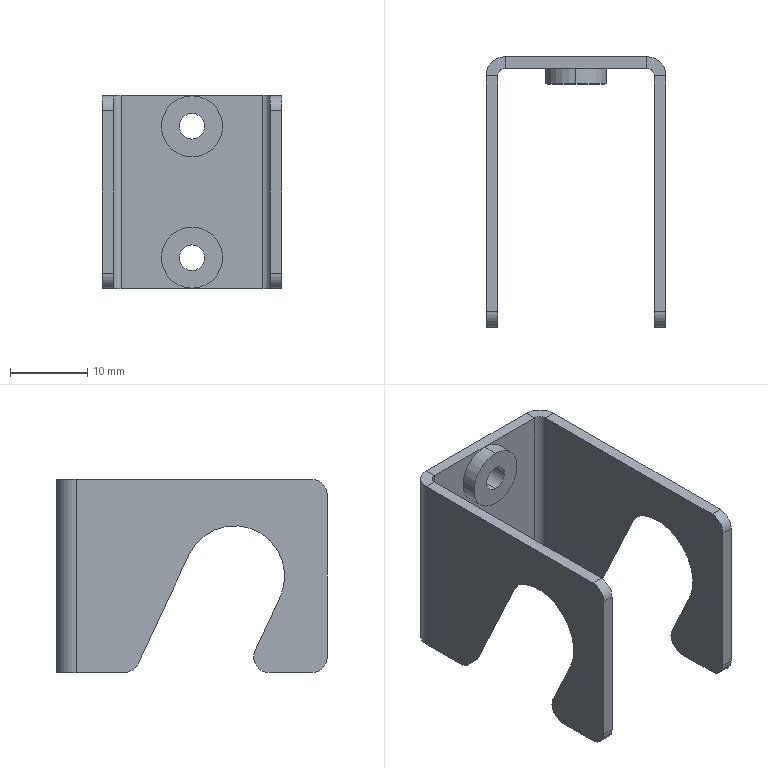Part | SolidWorks | features BaseBody 1 | 1 solid | 48 faces | box 23.3 x 35 x 25 mm | volume 2716 mm3 | plane 26 | cylinder 22 | commonest cylinder face diameters 4 x8 3.3 x4 7.9 x4 2 x2 5 x2 13 x2
STEP:
#1=CARTESIAN_POINT('',(0.,0.,10.15));
#2=VERTEX_POINT('',#1);
#3=CARTESIAN_POINT('',(0.,-3.5,10.15));
#4=VERTEX_POINT('',#3);
#5=CARTESIAN_POINT('',(0.,-3.5,10.15));
#6=DIRECTION('',(0.,-1.,0.));
#7=VECTOR('',#6,1000.);
#8=LINE('',#5,#7);
#9=EDGE_CURVE('',#2,#4,#8,.T.);
#10=ORIENTED_EDGE('',*,*,#9,.F.);
#11=CARTESIAN_POINT('',(0.,0.,6.85));
#12=VERTEX_POINT('',#11);
#13=CARTESIAN_POINT('',(0.,0.,8.5));
#14=DIRECTION('',(0.,-1.,0.));
#15=DIRECTION('',(0.,0.,-1.));
#16=AXIS2_PLACEMENT_3D('',#13,#14,#15);
#17=CIRCLE('',#16,1.65);
#18=EDGE_CURVE('',#12,#2,#17,.T.);
#19=ORIENTED_EDGE('',*,*,#18,.F.);
#20=CARTESIAN_POINT('',(0.,-3.5,6.85));
#21=VERTEX_POINT('',#20);
#22=CARTESIAN_POINT('',(0.,-3.5,6.85));
#23=DIRECTION('',(0.,-1.,0.));
#24=VECTOR('',#23,1000.);
#25=LINE('',#22,#24);
#26=EDGE_CURVE('',#12,#21,#25,.T.);
#27=ORIENTED_EDGE('',*,*,#26,.T.);
#28=CARTESIAN_POINT('',(0.,-3.5,8.5));
#29=DIRECTION('',(0.,-1.,0.));
#30=DIRECTION('',(0.,0.,-1.));
#31=AXIS2_PLACEMENT_3D('',#28,#29,#30);
#32=CIRCLE('',#31,1.65);
#33=EDGE_CURVE('',#21,#4,#32,.T.);
#34=ORIENTED_EDGE('',*,*,#33,.T.);
#35=EDGE_LOOP('',(#10,#19,#27,#34));
#36=FACE_OUTER_BOUND('',#35,.T.);
#37=CARTESIAN_POINT('',(0.,-3.5,8.5));
#38=DIRECTION('',(0.,-1.,0.));
#39=DIRECTION('',(0.,0.,-1.));
#40=AXIS2_PLACEMENT_3D('',#37,#38,#39);
#41=CYLINDRICAL_SURFACE('',#40,1.65);
#42=ADVANCED_FACE('',(#36),#41,.F.);
#43=CARTESIAN_POINT('',(0.,0.,-6.85));
#44=VERTEX_POINT('',#43);
#45=CARTESIAN_POINT('',(0.,-3.5,-6.85));
#46=VERTEX_POINT('',#45);
#47=CARTESIAN_POINT('',(0.,-3.5,-6.85));
#48=DIRECTION('',(0.,-1.,0.));
#49=VECTOR('',#48,1000.);
#50=LINE('',#47,#49);
#51=EDGE_CURVE('',#44,#46,#50,.T.);
#52=ORIENTED_EDGE('',*,*,#51,.F.);
#53=CARTESIAN_POINT('',(0.,0.,-10.15));
#54=VERTEX_POINT('',#53);
#55=CARTESIAN_POINT('',(0.,0.,-8.5));
#56=DIRECTION('',(0.,-1.,0.));
#57=DIRECTION('',(0.,0.,-1.));
#58=AXIS2_PLACEMENT_3D('',#55,#56,#57);
#59=CIRCLE('',#58,1.65);
#60=EDGE_CURVE('',#54,#44,#59,.T.);
#61=ORIENTED_EDGE('',*,*,#60,.F.);
#62=CARTESIAN_POINT('',(0.,-3.5,-10.15));
#63=VERTEX_POINT('',#62);
#64=CARTESIAN_POINT('',(0.,-3.5,-10.15));
#65=DIRECTION('',(0.,-1.,0.));
#66=VECTOR('',#65,1000.);
#67=LINE('',#64,#66);
#68=EDGE_CURVE('',#54,#63,#67,.T.);
#69=ORIENTED_EDGE('',*,*,#68,.T.);
#70=CARTESIAN_POINT('',(0.,-3.5,-8.5));
#71=DIRECTION('',(0.,-1.,0.));
#72=DIRECTION('',(0.,0.,-1.));
#73=AXIS2_PLACEMENT_3D('',#70,#71,#72);
#74=CIRCLE('',#73,1.65);
#75=EDGE_CURVE('',#63,#46,#74,.T.);
#76=ORIENTED_EDGE('',*,*,#75,.T.);
#77=EDGE_LOOP('',(#52,#61,#69,#76));
#78=FACE_OUTER_BOUND('',#77,.T.);
#79=CARTESIAN_POINT('',(0.,-3.5,-8.5));
#80=DIRECTION('',(0.,-1.,0.));
#81=DIRECTION('',(0.,0.,-1.));
#82=AXIS2_PLACEMENT_3D('',#79,#80,#81);
#83=CYLINDRICAL_SURFACE('',#82,1.65);
#84=ADVANCED_FACE('',(#78),#83,.F.);
#85=CARTESIAN_POINT('',(0.,-3.5,-12.45));
#86=VERTEX_POINT('',#85);
#87=CARTESIAN_POINT('',(0.,-1.5,-12.45));
#88=VERTEX_POINT('',#87);
#89=CARTESIAN_POINT('',(0.,-3.5,-12.45));
#90=DIRECTION('',(0.,1.,0.));
#91=VECTOR('',#90,1000.);
#92=LINE('',#89,#91);
#93=EDGE_CURVE('',#86,#88,#92,.T.);
#94=ORIENTED_EDGE('',*,*,#93,.F.);
#95=CARTESIAN_POINT('',(0.,-3.5,-4.55));
#96=VERTEX_POINT('',#95);
#97=CARTESIAN_POINT('',(0.,-3.5,-8.5));
#98=DIRECTION('',(0.,-1.,0.));
#99=DIRECTION('',(0.,0.,1.));
#100=AXIS2_PLACEMENT_3D('',#97,#98,#99);
#101=CIRCLE('',#100,3.95);
#102=EDGE_CURVE('',#96,#86,#101,.T.);
#103=ORIENTED_EDGE('',*,*,#102,.F.);
#104=CARTESIAN_POINT('',(0.,-1.5,-4.55));
#105=VERTEX_POINT('',#104);
#106=CARTESIAN_POINT('',(0.,-3.5,-4.55));
#107=DIRECTION('',(0.,1.,0.));
#108=VECTOR('',#107,1000.);
#109=LINE('',#106,#108);
#110=EDGE_CURVE('',#96,#105,#109,.T.);
#111=ORIENTED_EDGE('',*,*,#110,.T.);
#112=CARTESIAN_POINT('',(0.,-1.5,-8.5));
#113=DIRECTION('',(0.,-1.,0.));
#114=DIRECTION('',(0.,0.,1.));
#115=AXIS2_PLACEMENT_3D('',#112,#113,#114);
#116=CIRCLE('',#115,3.95);
#117=EDGE_CURVE('',#105,#88,#116,.T.);
#118=ORIENTED_EDGE('',*,*,#117,.T.);
#119=EDGE_LOOP('',(#94,#103,#111,#118));
#120=FACE_OUTER_BOUND('',#119,.T.);
#121=CARTESIAN_POINT('',(0.,-3.5,-8.5));
#122=DIRECTION('',(0.,1.,0.));
#123=DIRECTION('',(0.,0.,1.));
#124=AXIS2_PLACEMENT_3D('',#121,#122,#123);
#125=CYLINDRICAL_SURFACE('',#124,3.95);
#126=ADVANCED_FACE('',(#120),#125,.T.);
#127=ORIENTED_EDGE('',*,*,#33,.F.);
#128=CARTESIAN_POINT('',(0.,-3.5,8.5));
#129=DIRECTION('',(0.,-1.,0.));
#130=DIRECTION('',(0.,0.,-1.));
#131=AXIS2_PLACEMENT_3D('',#128,#129,#130);
#132=CIRCLE('',#131,1.65);
#133=EDGE_CURVE('',#4,#21,#132,.T.);
#134=ORIENTED_EDGE('',*,*,#133,.F.);
#135=EDGE_LOOP('',(#127,#134));
#136=FACE_BOUND('',#135,.T.);
#137=CARTESIAN_POINT('',(0.,-3.5,12.45));
#138=VERTEX_POINT('',#137);
#139=CARTESIAN_POINT('',(0.,-3.5,4.55));
#140=VERTEX_POINT('',#139);
#141=CARTESIAN_POINT('',(0.,-3.5,8.5));
#142=DIRECTION('',(0.,-1.,0.));
#143=DIRECTION('',(0.,0.,-1.));
#144=AXIS2_PLACEMENT_3D('',#141,#142,#143);
#145=CIRCLE('',#144,3.95);
#146=EDGE_CURVE('',#138,#140,#145,.T.);
#147=ORIENTED_EDGE('',*,*,#146,.T.);
#148=CARTESIAN_POINT('',(0.,-3.5,8.5));
#149=DIRECTION('',(0.,-1.,0.));
#150=DIRECTION('',(0.,0.,-1.));
#151=AXIS2_PLACEMENT_3D('',#148,#149,#150);
#152=CIRCLE('',#151,3.95);
#153=EDGE_CURVE('',#140,#138,#152,.T.);
#154=ORIENTED_EDGE('',*,*,#153,.T.);
#155=EDGE_LOOP('',(#147,#154));
#156=FACE_OUTER_BOUND('',#155,.T.);
#157=CARTESIAN_POINT('',(0.,-3.5,8.5));
#158=DIRECTION('',(0.,-1.,0.));
#159=DIRECTION('',(0.,0.,-1.));
#160=AXIS2_PLACEMENT_3D('',#157,#158,#159);
#161=PLANE('',#160);
#162=ADVANCED_FACE('',(#136,#156),#161,.T.);
#163=CARTESIAN_POINT('',(0.,-1.5,4.55));
#164=VERTEX_POINT('',#163);
#165=CARTESIAN_POINT('',(0.,-3.5,4.55));
#166=DIRECTION('',(0.,1.,0.));
#167=VECTOR('',#166,1000.);
#168=LINE('',#165,#167);
#169=EDGE_CURVE('',#140,#164,#168,.T.);
#170=ORIENTED_EDGE('',*,*,#169,.F.);
#171=ORIENTED_EDGE('',*,*,#146,.F.);
#172=CARTESIAN_POINT('',(0.,-1.5,12.45));
#173=VERTEX_POINT('',#172);
#174=CARTESIAN_POINT('',(0.,-3.5,12.45));
#175=DIRECTION('',(0.,1.,0.));
#176=VECTOR('',#175,1000.);
#177=LINE('',#174,#176);
#178=EDGE_CURVE('',#138,#173,#177,.T.);
#179=ORIENTED_EDGE('',*,*,#178,.T.);
#180=CARTESIAN_POINT('',(0.,-1.5,8.5));
#181=DIRECTION('',(0.,-1.,0.));
#182=DIRECTION('',(0.,0.,1.));
#183=AXIS2_PLACEMENT_3D('',#180,#181,#182);
#184=CIRCLE('',#183,3.95);
#185=EDGE_CURVE('',#173,#164,#184,.T.);
#186=ORIENTED_EDGE('',*,*,#185,.T.);
#187=EDGE_LOOP('',(#170,#171,#179,#186));
#188=FACE_OUTER_BOUND('',#187,.T.);
#189=CARTESIAN_POINT('',(0.,-3.5,8.5));
#190=DIRECTION('',(0.,1.,0.));
#191=DIRECTION('',(0.,0.,1.));
#192=AXIS2_PLACEMENT_3D('',#189,#190,#191);
#193=CYLINDRICAL_SURFACE('',#192,3.95);
#194=ADVANCED_FACE('',(#188),#193,.T.);
#195=CARTESIAN_POINT('',(11.65,-27.483,-12.5));
#196=VERTEX_POINT('',#195);
#197=CARTESIAN_POINT('',(11.65,-25.67,-9.655));
#198=VERTEX_POINT('',#197);
#199=CARTESIAN_POINT('',(11.65,-27.483,-10.5));
#200=DIRECTION('',(1.,0.,0.));
#201=DIRECTION('',(0.,1.,0.));
#202=AXIS2_PLACEMENT_3D('',#199,#200,#201);
#203=CIRCLE('',#202,2.);
#204=EDGE_CURVE('',#196,#198,#203,.T.);
#205=ORIENTED_EDGE('',*,*,#204,.F.);
#206=CARTESIAN_POINT('',(10.15,-27.483,-12.5));
#207=VERTEX_POINT('',#206);
#208=CARTESIAN_POINT('',(11.65,-27.483,-12.5));
#209=DIRECTION('',(1.,0.,0.));
#210=VECTOR('',#209,1000.);
#211=LINE('',#208,#210);
#212=EDGE_CURVE('',#207,#196,#211,.T.);
#213=ORIENTED_EDGE('',*,*,#212,.F.);
#214=CARTESIAN_POINT('',(10.15,-25.67,-9.655));
#215=VERTEX_POINT('',#214);
#216=CARTESIAN_POINT('',(10.15,-27.483,-10.5));
#217=DIRECTION('',(-1.,0.,0.));
#218=DIRECTION('',(0.,1.,0.));
#219=AXIS2_PLACEMENT_3D('',#216,#217,#218);
#220=CIRCLE('',#219,2.);
#221=EDGE_CURVE('',#215,#207,#220,.T.);
#222=ORIENTED_EDGE('',*,*,#221,.F.);
#223=CARTESIAN_POINT('',(11.65,-25.67,-9.655));
#224=DIRECTION('',(-1.,0.,0.));
#225=VECTOR('',#224,1000.);
#226=LINE('',#223,#225);
#227=EDGE_CURVE('',#198,#215,#226,.T.);
#228=ORIENTED_EDGE('',*,*,#227,.F.);
#229=EDGE_LOOP('',(#205,#213,#222,#228));
#230=FACE_OUTER_BOUND('',#229,.T.);
#231=CARTESIAN_POINT('',(11.65,-27.483,-10.5));
#232=DIRECTION('',(-1.,0.,0.));
#233=DIRECTION('',(0.,-1.,0.));
#234=AXIS2_PLACEMENT_3D('',#231,#232,#233);
#235=CYLINDRICAL_SURFACE('',#234,2.);
#236=ADVANCED_FACE('',(#230),#235,.T.);
#237=CARTESIAN_POINT('',(-10.15,-27.483,-12.5));
#238=VERTEX_POINT('',#237);
#239=CARTESIAN_POINT('',(-10.15,-25.67,-9.655));
#240=VERTEX_POINT('',#239);
#241=CARTESIAN_POINT('',(-10.15,-27.483,-10.5));
#242=DIRECTION('',(1.,0.,0.));
#243=DIRECTION('',(0.,1.,0.));
#244=AXIS2_PLACEMENT_3D('',#241,#242,#243);
#245=CIRCLE('',#244,2.);
#246=EDGE_CURVE('',#238,#240,#245,.T.);
#247=ORIENTED_EDGE('',*,*,#246,.F.);
#248=CARTESIAN_POINT('',(-11.65,-27.483,-12.5));
#249=VERTEX_POINT('',#248);
#250=CARTESIAN_POINT('',(-11.65,-27.483,-12.5));
#251=DIRECTION('',(1.,0.,0.));
#252=VECTOR('',#251,1000.);
#253=LINE('',#250,#252);
#254=EDGE_CURVE('',#249,#238,#253,.T.);
#255=ORIENTED_EDGE('',*,*,#254,.F.);
#256=CARTESIAN_POINT('',(-11.65,-25.67,-9.655));
#257=VERTEX_POINT('',#256);
#258=CARTESIAN_POINT('',(-11.65,-27.483,-10.5));
#259=DIRECTION('',(-1.,0.,0.));
#260=DIRECTION('',(0.,1.,0.));
#261=AXIS2_PLACEMENT_3D('',#258,#259,#260);
#262=CIRCLE('',#261,2.);
#263=EDGE_CURVE('',#257,#249,#262,.T.);
#264=ORIENTED_EDGE('',*,*,#263,.F.);
#265=CARTESIAN_POINT('',(-10.15,-25.67,-9.655));
#266=DIRECTION('',(-1.,0.,0.));
#267=VECTOR('',#266,1000.);
#268=LINE('',#265,#267);
#269=EDGE_CURVE('',#240,#257,#268,.T.);
#270=ORIENTED_EDGE('',*,*,#269,.F.);
#271=EDGE_LOOP('',(#247,#255,#264,#270));
#272=FACE_OUTER_BOUND('',#271,.T.);
#273=CARTESIAN_POINT('',(-10.15,-27.483,-10.5));
#274=DIRECTION('',(-1.,0.,0.));
#275=DIRECTION('',(0.,-1.,0.));
#276=AXIS2_PLACEMENT_3D('',#273,#274,#275);
#277=CYLINDRICAL_SURFACE('',#276,2.);
#278=ADVANCED_FACE('',(#272),#277,.T.);
#279=CARTESIAN_POINT('',(-11.65,-33.,-12.5));
#280=VERTEX_POINT('',#279);
#281=CARTESIAN_POINT('',(-11.65,-35.,-10.5));
#282=VERTEX_POINT('',#281);
#283=CARTESIAN_POINT('',(-11.65,-33.,-10.5));
#284=DIRECTION('',(-1.,0.,0.));
#285=DIRECTION('',(0.,1.,0.));
#286=AXIS2_PLACEMENT_3D('',#283,#284,#285);
#287=CIRCLE('',#286,2.);
#288=EDGE_CURVE('',#280,#282,#287,.T.);
#289=ORIENTED_EDGE('',*,*,#288,.F.);
#290=CARTESIAN_POINT('',(-10.15,-33.,-12.5));
#291=VERTEX_POINT('',#290);
#292=CARTESIAN_POINT('',(-11.65,-33.,-12.5));
#293=DIRECTION('',(-1.,0.,0.));
#294=VECTOR('',#293,1000.);
#295=LINE('',#292,#294);
#296=EDGE_CURVE('',#291,#280,#295,.T.);
#297=ORIENTED_EDGE('',*,*,#296,.F.);
#298=CARTESIAN_POINT('',(-10.15,-35.,-10.5));
#299=VERTEX_POINT('',#298);
#300=CARTESIAN_POINT('',(-10.15,-33.,-10.5));
#301=DIRECTION('',(1.,0.,0.));
#302=DIRECTION('',(0.,1.,0.));
#303=AXIS2_PLACEMENT_3D('',#300,#301,#302);
#304=CIRCLE('',#303,2.);
#305=EDGE_CURVE('',#299,#291,#304,.T.);
#306=ORIENTED_EDGE('',*,*,#305,.F.);
#307=CARTESIAN_POINT('',(-11.65,-35.,-10.5));
#308=DIRECTION('',(1.,0.,0.));
#309=VECTOR('',#308,1000.);
#310=LINE('',#307,#309);
#311=EDGE_CURVE('',#282,#299,#310,.T.);
#312=ORIENTED_EDGE('',*,*,#311,.F.);
#313=EDGE_LOOP('',(#289,#297,#306,#312));
#314=FACE_OUTER_BOUND('',#313,.T.);
#315=CARTESIAN_POINT('',(-11.65,-33.,-10.5));
#316=DIRECTION('',(1.,0.,0.));
#317=DIRECTION('',(0.,1.,0.));
#318=AXIS2_PLACEMENT_3D('',#315,#316,#317);
#319=CYLINDRICAL_SURFACE('',#318,2.);
#320=ADVANCED_FACE('',(#314),#319,.T.);
#321=CARTESIAN_POINT('',(11.65,-35.,-10.5));
#322=VERTEX_POINT('',#321);
#323=CARTESIAN_POINT('',(11.65,-33.,-12.5));
#324=VERTEX_POINT('',#323);
#325=CARTESIAN_POINT('',(11.65,-33.,-10.5));
#326=DIRECTION('',(1.,0.,0.));
#327=DIRECTION('',(0.,1.,0.));
#328=AXIS2_PLACEMENT_3D('',#325,#326,#327);
#329=CIRCLE('',#328,2.);
#330=EDGE_CURVE('',#322,#324,#329,.T.);
#331=ORIENTED_EDGE('',*,*,#330,.F.);
#332=CARTESIAN_POINT('',(10.15,-35.,-10.5));
#333=VERTEX_POINT('',#332);
#334=CARTESIAN_POINT('',(11.65,-35.,-10.5));
#335=DIRECTION('',(1.,0.,0.));
#336=VECTOR('',#335,1000.);
#337=LINE('',#334,#336);
#338=EDGE_CURVE('',#333,#322,#337,.T.);
#339=ORIENTED_EDGE('',*,*,#338,.F.);
#340=CARTESIAN_POINT('',(10.15,-33.,-12.5));
#341=VERTEX_POINT('',#340);
#342=CARTESIAN_POINT('',(10.15,-33.,-10.5));
#343=DIRECTION('',(-1.,0.,0.));
#344=DIRECTION('',(0.,1.,0.));
#345=AXIS2_PLACEMENT_3D('',#342,#343,#344);
#346=CIRCLE('',#345,2.);
#347=EDGE_CURVE('',#341,#333,#346,.T.);
#348=ORIENTED_EDGE('',*,*,#347,.F.);
#349=CARTESIAN_POINT('',(11.65,-33.,-12.5));
#350=DIRECTION('',(-1.,0.,0.));
#351=VECTOR('',#350,1000.);
#352=LINE('',#349,#351);
#353=EDGE_CURVE('',#324,#341,#352,.T.);
#354=ORIENTED_EDGE('',*,*,#353,.F.);
#355=EDGE_LOOP('',(#331,#339,#348,#354));
#356=FACE_OUTER_BOUND('',#355,.T.);
#357=CARTESIAN_POINT('',(11.65,-33.,-10.5));
#358=DIRECTION('',(-1.,0.,0.));
#359=DIRECTION('',(0.,-1.,0.));
#360=AXIS2_PLACEMENT_3D('',#357,#358,#359);
#361=CYLINDRICAL_SURFACE('',#360,2.);
#362=ADVANCED_FACE('',(#356),#361,.T.);
#363=CARTESIAN_POINT('',(-11.65,-35.,10.5));
#364=VERTEX_POINT('',#363);
#365=CARTESIAN_POINT('',(-11.65,-33.,12.5));
#366=VERTEX_POINT('',#365);
#367=CARTESIAN_POINT('',(-11.65,-33.,10.5));
#368=DIRECTION('',(-1.,0.,0.));
#369=DIRECTION('',(0.,1.,0.));
#370=AXIS2_PLACEMENT_3D('',#367,#368,#369);
#371=CIRCLE('',#370,2.);
#372=EDGE_CURVE('',#364,#366,#371,.T.);
#373=ORIENTED_EDGE('',*,*,#372,.F.);
#374=CARTESIAN_POINT('',(-10.15,-35.,10.5));
#375=VERTEX_POINT('',#374);
#376=CARTESIAN_POINT('',(-11.65,-35.,10.5));
#377=DIRECTION('',(-1.,0.,0.));
#378=VECTOR('',#377,1000.);
#379=LINE('',#376,#378);
#380=EDGE_CURVE('',#375,#364,#379,.T.);
#381=ORIENTED_EDGE('',*,*,#380,.F.);
#382=CARTESIAN_POINT('',(-10.15,-33.,12.5));
#383=VERTEX_POINT('',#382);
#384=CARTESIAN_POINT('',(-10.15,-33.,10.5));
#385=DIRECTION('',(1.,0.,0.));
#386=DIRECTION('',(0.,1.,0.));
#387=AXIS2_PLACEMENT_3D('',#384,#385,#386);
#388=CIRCLE('',#387,2.);
#389=EDGE_CURVE('',#383,#375,#388,.T.);
#390=ORIENTED_EDGE('',*,*,#389,.F.);
#391=CARTESIAN_POINT('',(-11.65,-33.,12.5));
#392=DIRECTION('',(1.,0.,0.));
#393=VECTOR('',#392,1000.);
#394=LINE('',#391,#393);
#395=EDGE_CURVE('',#366,#383,#394,.T.);
#396=ORIENTED_EDGE('',*,*,#395,.F.);
#397=EDGE_LOOP('',(#373,#381,#390,#396));
#398=FACE_OUTER_BOUND('',#397,.T.);
#399=CARTESIAN_POINT('',(-11.65,-33.,10.5));
#400=DIRECTION('',(1.,0.,0.));
#401=DIRECTION('',(0.,1.,0.));
#402=AXIS2_PLACEMENT_3D('',#399,#400,#401);
#403=CYLINDRICAL_SURFACE('',#402,2.);
#404=ADVANCED_FACE('',(#398),#403,.T.);
#405=CARTESIAN_POINT('',(11.65,-33.,12.5));
#406=VERTEX_POINT('',#405);
#407=CARTESIAN_POINT('',(11.65,-35.,10.5));
#408=VERTEX_POINT('',#407);
#409=CARTESIAN_POINT('',(11.65,-33.,10.5));
#410=DIRECTION('',(1.,0.,0.));
#411=DIRECTION('',(0.,1.,0.));
#412=AXIS2_PLACEMENT_3D('',#409,#410,#411);
#413=CIRCLE('',#412,2.);
#414=EDGE_CURVE('',#406,#408,#413,.T.);
#415=ORIENTED_EDGE('',*,*,#414,.F.);
#416=CARTESIAN_POINT('',(10.15,-33.,12.5));
#417=VERTEX_POINT('',#416);
#418=CARTESIAN_POINT('',(11.65,-33.,12.5));
#419=DIRECTION('',(1.,0.,0.));
#420=VECTOR('',#419,1000.);
#421=LINE('',#418,#420);
#422=EDGE_CURVE('',#417,#406,#421,.T.);
#423=ORIENTED_EDGE('',*,*,#422,.F.);
#424=CARTESIAN_POINT('',(10.15,-35.,10.5));
#425=VERTEX_POINT('',#424);
#426=CARTESIAN_POINT('',(10.15,-33.,10.5));
#427=DIRECTION('',(-1.,0.,0.));
#428=DIRECTION('',(0.,1.,0.));
#429=AXIS2_PLACEMENT_3D('',#426,#427,#428);
#430=CIRCLE('',#429,2.);
#431=EDGE_CURVE('',#425,#417,#430,.T.);
#432=ORIENTED_EDGE('',*,*,#431,.F.);
#433=CARTESIAN_POINT('',(11.65,-35.,10.5));
#434=DIRECTION('',(-1.,0.,0.));
#435=VECTOR('',#434,1000.);
#436=LINE('',#433,#435);
#437=EDGE_CURVE('',#408,#425,#436,.T.);
#438=ORIENTED_EDGE('',*,*,#437,.F.);
#439=EDGE_LOOP('',(#415,#423,#432,#438));
#440=FACE_OUTER_BOUND('',#439,.T.);
#441=CARTESIAN_POINT('',(11.65,-33.,10.5));
#442=DIRECTION('',(-1.,0.,0.));
#443=DIRECTION('',(0.,-1.,0.));
#444=AXIS2_PLACEMENT_3D('',#441,#442,#443);
#445=CYLINDRICAL_SURFACE('',#444,2.);
#446=ADVANCED_FACE('',(#440),#445,.T.);
#447=CARTESIAN_POINT('',(-10.15,-10.538,-11.345));
#448=VERTEX_POINT('',#447);
#449=CARTESIAN_POINT('',(-10.15,-8.726,-12.5));
#450=VERTEX_POINT('',#449);
#451=CARTESIAN_POINT('',(-10.15,-8.726,-10.5));
#452=DIRECTION('',(1.,0.,0.));
#453=DIRECTION('',(0.,1.,0.));
#454=AXIS2_PLACEMENT_3D('',#451,#452,#453);
#455=CIRCLE('',#454,2.);
#456=EDGE_CURVE('',#448,#450,#455,.T.);
#457=ORIENTED_EDGE('',*,*,#456,.F.);
#458=CARTESIAN_POINT('',(-11.65,-10.538,-11.345));
#459=VERTEX_POINT('',#458);
#460=CARTESIAN_POINT('',(-10.15,-10.538,-11.345));
#461=DIRECTION('',(1.,0.,0.));
#462=VECTOR('',#461,1000.);
#463=LINE('',#460,#462);
#464=EDGE_CURVE('',#459,#448,#463,.T.);
#465=ORIENTED_EDGE('',*,*,#464,.F.);
#466=CARTESIAN_POINT('',(-11.65,-8.726,-12.5));
#467=VERTEX_POINT('',#466);
#468=CARTESIAN_POINT('',(-11.65,-8.726,-10.5));
#469=DIRECTION('',(-1.,0.,0.));
#470=DIRECTION('',(0.,1.,0.));
#471=AXIS2_PLACEMENT_3D('',#468,#469,#470);
#472=CIRCLE('',#471,2.);
#473=EDGE_CURVE('',#467,#459,#472,.T.);
#474=ORIENTED_EDGE('',*,*,#473,.F.);
#475=CARTESIAN_POINT('',(-11.65,-8.726,-12.5));
#476=DIRECTION('',(-1.,0.,0.));
#477=VECTOR('',#476,1000.);
#478=LINE('',#475,#477);
#479=EDGE_CURVE('',#450,#467,#478,.T.);
#480=ORIENTED_EDGE('',*,*,#479,.F.);
#481=EDGE_LOOP('',(#457,#465,#474,#480));
#482=FACE_OUTER_BOUND('',#481,.T.);
#483=CARTESIAN_POINT('',(-11.65,-8.726,-10.5));
#484=DIRECTION('',(-1.,0.,0.));
#485=DIRECTION('',(0.,-1.,0.));
#486=AXIS2_PLACEMENT_3D('',#483,#484,#485);
#487=CYLINDRICAL_SURFACE('',#486,2.);
#488=ADVANCED_FACE('',(#482),#487,.T.);
#489=CARTESIAN_POINT('',(11.65,-10.538,-11.345));
#490=VERTEX_POINT('',#489);
#491=CARTESIAN_POINT('',(11.65,-8.726,-12.5));
#492=VERTEX_POINT('',#491);
#493=CARTESIAN_POINT('',(11.65,-8.726,-10.5));
#494=DIRECTION('',(1.,0.,0.));
#495=DIRECTION('',(0.,1.,0.));
#496=AXIS2_PLACEMENT_3D('',#493,#494,#495);
#497=CIRCLE('',#496,2.);
#498=EDGE_CURVE('',#490,#492,#497,.T.);
#499=ORIENTED_EDGE('',*,*,#498,.F.);
#500=CARTESIAN_POINT('',(10.15,-10.538,-11.345));
#501=VERTEX_POINT('',#500);
#502=CARTESIAN_POINT('',(11.65,-10.538,-11.345));
#503=DIRECTION('',(1.,0.,0.));
#504=VECTOR('',#503,1000.);
#505=LINE('',#502,#504);
#506=EDGE_CURVE('',#501,#490,#505,.T.);
#507=ORIENTED_EDGE('',*,*,#506,.F.);
#508=CARTESIAN_POINT('',(10.15,-8.726,-12.5));
#509=VERTEX_POINT('',#508);
#510=CARTESIAN_POINT('',(10.15,-8.726,-10.5));
#511=DIRECTION('',(-1.,0.,0.));
#512=DIRECTION('',(0.,1.,0.));
#513=AXIS2_PLACEMENT_3D('',#510,#511,#512);
#514=CIRCLE('',#513,2.);
#515=EDGE_CURVE('',#509,#501,#514,.T.);
#516=ORIENTED_EDGE('',*,*,#515,.F.);
#517=CARTESIAN_POINT('',(11.65,-8.726,-12.5));
#518=DIRECTION('',(-1.,0.,0.));
#519=VECTOR('',#518,1000.);
#520=LINE('',#517,#519);
#521=EDGE_CURVE('',#492,#509,#520,.T.);
#522=ORIENTED_EDGE('',*,*,#521,.F.);
#523=EDGE_LOOP('',(#499,#507,#516,#522));
#524=FACE_OUTER_BOUND('',#523,.T.);
#525=CARTESIAN_POINT('',(11.65,-8.726,-10.5));
#526=DIRECTION('',(-1.,0.,0.));
#527=DIRECTION('',(0.,-1.,0.));
#528=AXIS2_PLACEMENT_3D('',#525,#526,#527);
#529=CYLINDRICAL_SURFACE('',#528,2.);
#530=ADVANCED_FACE('',(#524),#529,.T.);
#531=CARTESIAN_POINT('',(11.65,-28.891,-2.747));
#532=VERTEX_POINT('',#531);
#533=CARTESIAN_POINT('',(11.65,-17.109,2.747));
#534=VERTEX_POINT('',#533);
#535=CARTESIAN_POINT('',(11.65,-23.,0.));
#536=DIRECTION('',(-1.,0.,0.));
#537=DIRECTION('',(0.,1.,0.));
#538=AXIS2_PLACEMENT_3D('',#535,#536,#537);
#539=CIRCLE('',#538,6.5);
#540=EDGE_CURVE('',#532,#534,#539,.T.);
#541=ORIENTED_EDGE('',*,*,#540,.F.);
#542=CARTESIAN_POINT('',(10.15,-28.891,-2.747));
#543=VERTEX_POINT('',#542);
#544=CARTESIAN_POINT('',(11.65,-28.891,-2.747));
#545=DIRECTION('',(-1.,0.,0.));
#546=VECTOR('',#545,1000.);
#547=LINE('',#544,#546);
#548=EDGE_CURVE('',#532,#543,#547,.T.);
#549=ORIENTED_EDGE('',*,*,#548,.T.);
#550=CARTESIAN_POINT('',(10.15,-17.109,2.747));
#551=VERTEX_POINT('',#550);
#552=CARTESIAN_POINT('',(10.15,-23.,0.));
#553=DIRECTION('',(-1.,0.,0.));
#554=DIRECTION('',(0.,1.,0.));
#555=AXIS2_PLACEMENT_3D('',#552,#553,#554);
#556=CIRCLE('',#555,6.5);
#557=EDGE_CURVE('',#543,#551,#556,.T.);
#558=ORIENTED_EDGE('',*,*,#557,.T.);
#559=CARTESIAN_POINT('',(11.65,-17.109,2.747));
#560=DIRECTION('',(-1.,0.,0.));
#561=VECTOR('',#560,1000.);
#562=LINE('',#559,#561);
#563=EDGE_CURVE('',#534,#551,#562,.T.);
#564=ORIENTED_EDGE('',*,*,#563,.F.);
#565=EDGE_LOOP('',(#541,#549,#558,#564));
#566=FACE_OUTER_BOUND('',#565,.T.);
#567=CARTESIAN_POINT('',(11.65,-23.,0.));
#568=DIRECTION('',(1.,0.,0.));
#569=DIRECTION('',(0.,1.,0.));
#570=AXIS2_PLACEMENT_3D('',#567,#568,#569);
#571=CYLINDRICAL_SURFACE('',#570,6.5);
#572=ADVANCED_FACE('',(#566),#571,.F.);
#573=CARTESIAN_POINT('',(10.15,-13.002,-6.062));
#574=DIRECTION('',(0.,0.4226,-0.9063));
#575=VECTOR('',#574,1000.);
#576=LINE('',#573,#575);
#577=EDGE_CURVE('',#551,#501,#576,.T.);
#578=ORIENTED_EDGE('',*,*,#577,.T.);
#579=ORIENTED_EDGE('',*,*,#506,.T.);
#580=CARTESIAN_POINT('',(11.65,-13.002,-6.062));
#581=DIRECTION('',(0.,0.4226,-0.9063));
#582=VECTOR('',#581,1000.);
#583=LINE('',#580,#582);
#584=EDGE_CURVE('',#534,#490,#583,.T.);
#585=ORIENTED_EDGE('',*,*,#584,.F.);
#586=ORIENTED_EDGE('',*,*,#563,.T.);
#587=EDGE_LOOP('',(#578,#579,#585,#586));
#588=FACE_OUTER_BOUND('',#587,.T.);
#589=CARTESIAN_POINT('',(11.65,-13.002,-6.062));
#590=DIRECTION('',(0.,-0.9063,-0.4226));
#591=DIRECTION('',(0.,0.4226,-0.9063));
#592=AXIS2_PLACEMENT_3D('',#589,#590,#591);
#593=PLANE('',#592);
#594=ADVANCED_FACE('',(#588),#593,.T.);
#595=CARTESIAN_POINT('',(11.65,-24.784,-11.556));
#596=DIRECTION('',(0.,-0.4226,0.9063));
#597=VECTOR('',#596,1000.);
#598=LINE('',#595,#597);
#599=EDGE_CURVE('',#198,#532,#598,.T.);
#600=ORIENTED_EDGE('',*,*,#599,.F.);
#601=ORIENTED_EDGE('',*,*,#227,.T.);
#602=CARTESIAN_POINT('',(10.15,-24.784,-11.556));
#603=DIRECTION('',(0.,-0.4226,0.9063));
#604=VECTOR('',#603,1000.);
#605=LINE('',#602,#604);
#606=EDGE_CURVE('',#215,#543,#605,.T.);
#607=ORIENTED_EDGE('',*,*,#606,.T.);
#608=ORIENTED_EDGE('',*,*,#548,.F.);
#609=EDGE_LOOP('',(#600,#601,#607,#608));
#610=FACE_OUTER_BOUND('',#609,.T.);
#611=CARTESIAN_POINT('',(11.65,-24.784,-11.556));
#612=DIRECTION('',(0.,0.9063,0.4226));
#613=DIRECTION('',(1.,0.,0.));
#614=AXIS2_PLACEMENT_3D('',#611,#612,#613);
#615=PLANE('',#614);
#616=ADVANCED_FACE('',(#610),#615,.T.);
#617=CARTESIAN_POINT('',(-10.15,-28.891,-2.747));
#618=VERTEX_POINT('',#617);
#619=CARTESIAN_POINT('',(-10.15,-24.784,-11.556));
#620=DIRECTION('',(0.,-0.4226,0.9063));
#621=VECTOR('',#620,1000.);
#622=LINE('',#619,#621);
#623=EDGE_CURVE('',#240,#618,#622,.T.);
#624=ORIENTED_EDGE('',*,*,#623,.F.);
#625=ORIENTED_EDGE('',*,*,#269,.T.);
#626=CARTESIAN_POINT('',(-11.65,-28.891,-2.747));
#627=VERTEX_POINT('',#626);
#628=CARTESIAN_POINT('',(-11.65,-24.784,-11.556));
#629=DIRECTION('',(0.,-0.4226,0.9063));
#630=VECTOR('',#629,1000.);
#631=LINE('',#628,#630);
#632=EDGE_CURVE('',#257,#627,#631,.T.);
#633=ORIENTED_EDGE('',*,*,#632,.T.);
#634=CARTESIAN_POINT('',(-10.15,-28.891,-2.747));
#635=DIRECTION('',(-1.,0.,0.));
#636=VECTOR('',#635,1000.);
#637=LINE('',#634,#636);
#638=EDGE_CURVE('',#618,#627,#637,.T.);
#639=ORIENTED_EDGE('',*,*,#638,.F.);
#640=EDGE_LOOP('',(#624,#625,#633,#639));
#641=FACE_OUTER_BOUND('',#640,.T.);
#642=CARTESIAN_POINT('',(-10.15,-24.784,-11.556));
#643=DIRECTION('',(0.,0.9063,0.4226));
#644=DIRECTION('',(1.,0.,0.));
#645=AXIS2_PLACEMENT_3D('',#642,#643,#644);
#646=PLANE('',#645);
#647=ADVANCED_FACE('',(#641),#646,.T.);
#648=CARTESIAN_POINT('',(-10.15,-17.109,2.747));
#649=VERTEX_POINT('',#648);
#650=CARTESIAN_POINT('',(-11.65,-17.109,2.747));
#651=VERTEX_POINT('',#650);
#652=CARTESIAN_POINT('',(-10.15,-17.109,2.747));
#653=DIRECTION('',(-1.,0.,0.));
#654=VECTOR('',#653,1000.);
#655=LINE('',#652,#654);
#656=EDGE_CURVE('',#649,#651,#655,.T.);
#657=ORIENTED_EDGE('',*,*,#656,.F.);
#658=CARTESIAN_POINT('',(-10.15,-23.,0.));
#659=DIRECTION('',(-1.,0.,0.));
#660=DIRECTION('',(0.,1.,0.));
#661=AXIS2_PLACEMENT_3D('',#658,#659,#660);
#662=CIRCLE('',#661,6.5);
#663=EDGE_CURVE('',#618,#649,#662,.T.);
#664=ORIENTED_EDGE('',*,*,#663,.F.);
#665=ORIENTED_EDGE('',*,*,#638,.T.);
#666=CARTESIAN_POINT('',(-11.65,-23.,0.));
#667=DIRECTION('',(-1.,0.,0.));
#668=DIRECTION('',(0.,1.,0.));
#669=AXIS2_PLACEMENT_3D('',#666,#667,#668);
#670=CIRCLE('',#669,6.5);
#671=EDGE_CURVE('',#627,#651,#670,.T.);
#672=ORIENTED_EDGE('',*,*,#671,.T.);
#673=EDGE_LOOP('',(#657,#664,#665,#672));
#674=FACE_OUTER_BOUND('',#673,.T.);
#675=CARTESIAN_POINT('',(-10.15,-23.,0.));
#676=DIRECTION('',(1.,0.,0.));
#677=DIRECTION('',(0.,1.,0.));
#678=AXIS2_PLACEMENT_3D('',#675,#676,#677);
#679=CYLINDRICAL_SURFACE('',#678,6.5);
#680=ADVANCED_FACE('',(#674),#679,.F.);
#681=CARTESIAN_POINT('',(-11.65,-13.002,-6.062));
#682=DIRECTION('',(0.,0.4226,-0.9063));
#683=VECTOR('',#682,1000.);
#684=LINE('',#681,#683);
#685=EDGE_CURVE('',#651,#459,#684,.T.);
#686=ORIENTED_EDGE('',*,*,#685,.T.);
#687=ORIENTED_EDGE('',*,*,#464,.T.);
#688=CARTESIAN_POINT('',(-10.15,-13.002,-6.062));
#689=DIRECTION('',(0.,0.4226,-0.9063));
#690=VECTOR('',#689,1000.);
#691=LINE('',#688,#690);
#692=EDGE_CURVE('',#649,#448,#691,.T.);
#693=ORIENTED_EDGE('',*,*,#692,.F.);
#694=ORIENTED_EDGE('',*,*,#656,.T.);
#695=EDGE_LOOP('',(#686,#687,#693,#694));
#696=FACE_OUTER_BOUND('',#695,.T.);
#697=CARTESIAN_POINT('',(-10.15,-13.002,-6.062));
#698=DIRECTION('',(0.,-0.9063,-0.4226));
#699=DIRECTION('',(0.,0.4226,-0.9063));
#700=AXIS2_PLACEMENT_3D('',#697,#698,#699);
#701=PLANE('',#700);
#702=ADVANCED_FACE('',(#696),#701,.T.);
#703=CARTESIAN_POINT('',(-10.15,-35.,0.));
#704=DIRECTION('',(0.,0.,-1.));
#705=VECTOR('',#704,1000.);
#706=LINE('',#703,#705);
#707=EDGE_CURVE('',#375,#299,#706,.T.);
#708=ORIENTED_EDGE('',*,*,#707,.F.);
#709=ORIENTED_EDGE('',*,*,#380,.T.);
#710=CARTESIAN_POINT('',(-11.65,-35.,12.5));
#711=DIRECTION('',(0.,0.,-1.));
#712=VECTOR('',#711,1000.);
#713=LINE('',#710,#712);
#714=EDGE_CURVE('',#364,#282,#713,.T.);
#715=ORIENTED_EDGE('',*,*,#714,.T.);
#716=ORIENTED_EDGE('',*,*,#311,.T.);
#717=EDGE_LOOP('',(#708,#709,#715,#716));
#718=FACE_OUTER_BOUND('',#717,.T.);
#719=CARTESIAN_POINT('',(-11.65,-35.,12.5));
#720=DIRECTION('',(0.,-1.,0.));
#721=DIRECTION('',(-1.,0.,0.));
#722=AXIS2_PLACEMENT_3D('',#719,#720,#721);
#723=PLANE('',#722);
#724=ADVANCED_FACE('',(#718),#723,.T.);
#725=CARTESIAN_POINT('',(-11.65,-2.5,12.5));
#726=VERTEX_POINT('',#725);
#727=CARTESIAN_POINT('',(-11.65,-1.5,12.5));
#728=DIRECTION('',(0.,-1.,0.));
#729=VECTOR('',#728,1000.);
#730=LINE('',#727,#729);
#731=EDGE_CURVE('',#726,#366,#730,.T.);
#732=ORIENTED_EDGE('',*,*,#731,.T.);
#733=ORIENTED_EDGE('',*,*,#395,.T.);
#734=CARTESIAN_POINT('',(-10.15,-2.5,12.5));
#735=VERTEX_POINT('',#734);
#736=CARTESIAN_POINT('',(-10.15,0.,12.5));
#737=DIRECTION('',(0.,-1.,0.));
#738=VECTOR('',#737,1000.);
#739=LINE('',#736,#738);
#740=EDGE_CURVE('',#735,#383,#739,.T.);
#741=ORIENTED_EDGE('',*,*,#740,.F.);
#742=CARTESIAN_POINT('',(-11.65,-2.5,12.5));
#743=DIRECTION('',(-1.,0.,0.));
#744=VECTOR('',#743,1000.);
#745=LINE('',#742,#744);
#746=EDGE_CURVE('',#735,#726,#745,.T.);
#747=ORIENTED_EDGE('',*,*,#746,.T.);
#748=EDGE_LOOP('',(#732,#733,#741,#747));
#749=FACE_OUTER_BOUND('',#748,.T.);
#750=CARTESIAN_POINT('',(-11.65,-1.5,12.5));
#751=DIRECTION('',(0.,0.,1.));
#752=DIRECTION('',(1.,0.,0.));
#753=AXIS2_PLACEMENT_3D('',#750,#751,#752);
#754=PLANE('',#753);
#755=ADVANCED_FACE('',(#749),#754,.T.);
#756=CARTESIAN_POINT('',(-9.15,-1.5,-12.5));
#757=VERTEX_POINT('',#756);
#758=CARTESIAN_POINT('',(-9.15,-1.5,12.5));
#759=VERTEX_POINT('',#758);
#760=CARTESIAN_POINT('',(-9.15,-1.5,-12.5));
#761=DIRECTION('',(0.,0.,1.));
#762=VECTOR('',#761,1000.);
#763=LINE('',#760,#762);
#764=EDGE_CURVE('',#757,#759,#763,.T.);
#765=ORIENTED_EDGE('',*,*,#764,.T.);
#766=CARTESIAN_POINT('',(-9.15,-2.5,12.5));
#767=DIRECTION('',(0.,0.,1.));
#768=DIRECTION('',(-1.,0.,0.));
#769=AXIS2_PLACEMENT_3D('',#766,#767,#768);
#770=CIRCLE('',#769,1.);
#771=EDGE_CURVE('',#759,#735,#770,.T.);
#772=ORIENTED_EDGE('',*,*,#771,.T.);
#773=CARTESIAN_POINT('',(-10.15,-2.5,-12.5));
#774=VERTEX_POINT('',#773);
#775=CARTESIAN_POINT('',(-10.15,-2.5,12.5));
#776=DIRECTION('',(0.,0.,-1.));
#777=VECTOR('',#776,1000.);
#778=LINE('',#775,#777);
#779=EDGE_CURVE('',#735,#774,#778,.T.);
#780=ORIENTED_EDGE('',*,*,#779,.T.);
#781=CARTESIAN_POINT('',(-9.15,-2.5,-12.5));
#782=DIRECTION('',(0.,0.,-1.));
#783=DIRECTION('',(-1.,0.,0.));
#784=AXIS2_PLACEMENT_3D('',#781,#782,#783);
#785=CIRCLE('',#784,1.);
#786=EDGE_CURVE('',#774,#757,#785,.T.);
#787=ORIENTED_EDGE('',*,*,#786,.T.);
#788=EDGE_LOOP('',(#765,#772,#780,#787));
#789=FACE_OUTER_BOUND('',#788,.T.);
#790=CARTESIAN_POINT('',(-9.15,-2.5,-12.5));
#791=DIRECTION('',(0.,0.,-1.));
#792=DIRECTION('',(-1.,0.,0.));
#793=AXIS2_PLACEMENT_3D('',#790,#791,#792);
#794=CYLINDRICAL_SURFACE('',#793,1.);
#795=ADVANCED_FACE('',(#789),#794,.F.);
#796=CARTESIAN_POINT('',(-9.15,0.,-12.5));
#797=VERTEX_POINT('',#796);
#798=CARTESIAN_POINT('',(-9.15,0.,12.5));
#799=VERTEX_POINT('',#798);
#800=CARTESIAN_POINT('',(-9.15,0.,-12.5));
#801=DIRECTION('',(0.,0.,1.));
#802=VECTOR('',#801,1000.);
#803=LINE('',#800,#802);
#804=EDGE_CURVE('',#797,#799,#803,.T.);
#805=ORIENTED_EDGE('',*,*,#804,.F.);
#806=CARTESIAN_POINT('',(-11.65,-2.5,-12.5));
#807=VERTEX_POINT('',#806);
#808=CARTESIAN_POINT('',(-9.15,-2.5,-12.5));
#809=DIRECTION('',(0.,0.,-1.));
#810=DIRECTION('',(-1.,0.,0.));
#811=AXIS2_PLACEMENT_3D('',#808,#809,#810);
#812=CIRCLE('',#811,2.5);
#813=EDGE_CURVE('',#807,#797,#812,.T.);
#814=ORIENTED_EDGE('',*,*,#813,.F.);
#815=CARTESIAN_POINT('',(-11.65,-2.5,12.5));
#816=DIRECTION('',(0.,0.,1.));
#817=VECTOR('',#816,1000.);
#818=LINE('',#815,#817);
#819=EDGE_CURVE('',#807,#726,#818,.T.);
#820=ORIENTED_EDGE('',*,*,#819,.T.);
#821=CARTESIAN_POINT('',(-9.15,-2.5,12.5));
#822=DIRECTION('',(0.,0.,1.));
#823=DIRECTION('',(-1.,0.,0.));
#824=AXIS2_PLACEMENT_3D('',#821,#822,#823);
#825=CIRCLE('',#824,2.5);
#826=EDGE_CURVE('',#799,#726,#825,.T.);
#827=ORIENTED_EDGE('',*,*,#826,.F.);
#828=EDGE_LOOP('',(#805,#814,#820,#827));
#829=FACE_OUTER_BOUND('',#828,.T.);
#830=CARTESIAN_POINT('',(-9.15,-2.5,-12.5));
#831=DIRECTION('',(0.,0.,-1.));
#832=DIRECTION('',(-1.,0.,0.));
#833=AXIS2_PLACEMENT_3D('',#830,#831,#832);
#834=CYLINDRICAL_SURFACE('',#833,2.5);
#835=ADVANCED_FACE('',(#829),#834,.T.);
#836=ORIENTED_EDGE('',*,*,#786,.F.);
#837=CARTESIAN_POINT('',(-10.15,-2.5,-12.5));
#838=DIRECTION('',(-1.,0.,0.));
#839=VECTOR('',#838,1000.);
#840=LINE('',#837,#839);
#841=EDGE_CURVE('',#774,#807,#840,.T.);
#842=ORIENTED_EDGE('',*,*,#841,.T.);
#843=ORIENTED_EDGE('',*,*,#813,.T.);
#844=CARTESIAN_POINT('',(-9.15,-1.5,-12.5));
#845=DIRECTION('',(0.,1.,0.));
#846=VECTOR('',#845,1000.);
#847=LINE('',#844,#846);
#848=EDGE_CURVE('',#757,#797,#847,.T.);
#849=ORIENTED_EDGE('',*,*,#848,.F.);
#850=EDGE_LOOP('',(#836,#842,#843,#849));
#851=FACE_OUTER_BOUND('',#850,.T.);
#852=CARTESIAN_POINT('',(-9.15,-2.5,-12.5));
#853=DIRECTION('',(0.,0.,1.));
#854=DIRECTION('',(1.,0.,0.));
#855=AXIS2_PLACEMENT_3D('',#852,#853,#854);
#856=PLANE('',#855);
#857=ADVANCED_FACE('',(#851),#856,.F.);
#858=ORIENTED_EDGE('',*,*,#746,.F.);
#859=ORIENTED_EDGE('',*,*,#771,.F.);
#860=CARTESIAN_POINT('',(-9.15,-1.5,12.5));
#861=DIRECTION('',(0.,1.,0.));
#862=VECTOR('',#861,1000.);
#863=LINE('',#860,#862);
#864=EDGE_CURVE('',#759,#799,#863,.T.);
#865=ORIENTED_EDGE('',*,*,#864,.T.);
#866=ORIENTED_EDGE('',*,*,#826,.T.);
#867=EDGE_LOOP('',(#858,#859,#865,#866));
#868=FACE_OUTER_BOUND('',#867,.T.);
#869=CARTESIAN_POINT('',(-9.15,-2.5,12.5));
#870=DIRECTION('',(0.,0.,1.));
#871=DIRECTION('',(1.,0.,0.));
#872=AXIS2_PLACEMENT_3D('',#869,#870,#871);
#873=PLANE('',#872);
#874=ADVANCED_FACE('',(#868),#873,.T.);
#875=CARTESIAN_POINT('',(11.65,-35.,12.5));
#876=DIRECTION('',(0.,0.,1.));
#877=VECTOR('',#876,1000.);
#878=LINE('',#875,#877);
#879=EDGE_CURVE('',#322,#408,#878,.T.);
#880=ORIENTED_EDGE('',*,*,#879,.T.);
#881=ORIENTED_EDGE('',*,*,#437,.T.);
#882=CARTESIAN_POINT('',(10.15,-35.,0.));
#883=DIRECTION('',(0.,0.,1.));
#884=VECTOR('',#883,1000.);
#885=LINE('',#882,#884);
#886=EDGE_CURVE('',#333,#425,#885,.T.);
#887=ORIENTED_EDGE('',*,*,#886,.F.);
#888=ORIENTED_EDGE('',*,*,#338,.T.);
#889=EDGE_LOOP('',(#880,#881,#887,#888));
#890=FACE_OUTER_BOUND('',#889,.T.);
#891=CARTESIAN_POINT('',(11.65,-35.,12.5));
#892=DIRECTION('',(0.,-1.,0.));
#893=DIRECTION('',(0.,0.,-1.));
#894=AXIS2_PLACEMENT_3D('',#891,#892,#893);
#895=PLANE('',#894);
#896=ADVANCED_FACE('',(#890),#895,.T.);
#897=CARTESIAN_POINT('',(10.15,-2.5,-12.5));
#898=VERTEX_POINT('',#897);
#899=CARTESIAN_POINT('',(10.15,0.,-12.5));
#900=DIRECTION('',(0.,-1.,0.));
#901=VECTOR('',#900,1000.);
#902=LINE('',#899,#901);
#903=EDGE_CURVE('',#898,#509,#902,.T.);
#904=ORIENTED_EDGE('',*,*,#903,.T.);
#905=ORIENTED_EDGE('',*,*,#515,.T.);
#906=ORIENTED_EDGE('',*,*,#577,.F.);
#907=ORIENTED_EDGE('',*,*,#557,.F.);
#908=ORIENTED_EDGE('',*,*,#606,.F.);
#909=ORIENTED_EDGE('',*,*,#221,.T.);
#910=CARTESIAN_POINT('',(10.15,0.,-12.5));
#911=DIRECTION('',(0.,-1.,0.));
#912=VECTOR('',#911,1000.);
#913=LINE('',#910,#912);
#914=EDGE_CURVE('',#207,#341,#913,.T.);
#915=ORIENTED_EDGE('',*,*,#914,.T.);
#916=ORIENTED_EDGE('',*,*,#347,.T.);
#917=ORIENTED_EDGE('',*,*,#886,.T.);
#918=ORIENTED_EDGE('',*,*,#431,.T.);
#919=CARTESIAN_POINT('',(10.15,-2.5,12.5));
#920=VERTEX_POINT('',#919);
#921=CARTESIAN_POINT('',(10.15,0.,12.5));
#922=DIRECTION('',(0.,1.,0.));
#923=VECTOR('',#922,1000.);
#924=LINE('',#921,#923);
#925=EDGE_CURVE('',#417,#920,#924,.T.);
#926=ORIENTED_EDGE('',*,*,#925,.T.);
#927=CARTESIAN_POINT('',(10.15,-2.5,-12.5));
#928=DIRECTION('',(0.,0.,1.));
#929=VECTOR('',#928,1000.);
#930=LINE('',#927,#929);
#931=EDGE_CURVE('',#898,#920,#930,.T.);
#932=ORIENTED_EDGE('',*,*,#931,.F.);
#933=EDGE_LOOP('',(#904,#905,#906,#907,#908,#909,#915,#916,#917,#918,#926,#932));
#934=FACE_OUTER_BOUND('',#933,.T.);
#935=CARTESIAN_POINT('',(10.15,0.,0.));
#936=DIRECTION('',(1.,0.,0.));
#937=DIRECTION('',(0.,1.,0.));
#938=AXIS2_PLACEMENT_3D('',#935,#936,#937);
#939=PLANE('',#938);
#940=ADVANCED_FACE('',(#934),#939,.F.);
#941=ORIENTED_EDGE('',*,*,#584,.T.);
#942=ORIENTED_EDGE('',*,*,#498,.T.);
#943=CARTESIAN_POINT('',(11.65,-2.5,-12.5));
#944=VERTEX_POINT('',#943);
#945=CARTESIAN_POINT('',(11.65,-35.,-12.5));
#946=DIRECTION('',(0.,-1.,0.));
#947=VECTOR('',#946,1000.);
#948=LINE('',#945,#947);
#949=EDGE_CURVE('',#944,#492,#948,.T.);
#950=ORIENTED_EDGE('',*,*,#949,.F.);
#951=CARTESIAN_POINT('',(11.65,-2.5,12.5));
#952=VERTEX_POINT('',#951);
#953=CARTESIAN_POINT('',(11.65,-2.5,0.));
#954=DIRECTION('',(0.,0.,1.));
#955=VECTOR('',#954,1000.);
#956=LINE('',#953,#955);
#957=EDGE_CURVE('',#944,#952,#956,.T.);
#958=ORIENTED_EDGE('',*,*,#957,.T.);
#959=CARTESIAN_POINT('',(11.65,-1.5,12.5));
#960=DIRECTION('',(0.,1.,0.));
#961=VECTOR('',#960,1000.);
#962=LINE('',#959,#961);
#963=EDGE_CURVE('',#406,#952,#962,.T.);
#964=ORIENTED_EDGE('',*,*,#963,.F.);
#965=ORIENTED_EDGE('',*,*,#414,.T.);
#966=ORIENTED_EDGE('',*,*,#879,.F.);
#967=ORIENTED_EDGE('',*,*,#330,.T.);
#968=CARTESIAN_POINT('',(11.65,-35.,-12.5));
#969=DIRECTION('',(0.,-1.,0.));
#970=VECTOR('',#969,1000.);
#971=LINE('',#968,#970);
#972=EDGE_CURVE('',#196,#324,#971,.T.);
#973=ORIENTED_EDGE('',*,*,#972,.F.);
#974=ORIENTED_EDGE('',*,*,#204,.T.);
#975=ORIENTED_EDGE('',*,*,#599,.T.);
#976=ORIENTED_EDGE('',*,*,#540,.T.);
#977=EDGE_LOOP('',(#941,#942,#950,#958,#964,#965,#966,#967,#973,#974,#975,#976));
#978=FACE_OUTER_BOUND('',#977,.T.);
#979=CARTESIAN_POINT('',(11.65,0.,0.));
#980=DIRECTION('',(1.,0.,0.));
#981=DIRECTION('',(0.,1.,0.));
#982=AXIS2_PLACEMENT_3D('',#979,#980,#981);
#983=PLANE('',#982);
#984=ADVANCED_FACE('',(#978),#983,.T.);
#985=ORIENTED_EDGE('',*,*,#925,.F.);
#986=ORIENTED_EDGE('',*,*,#422,.T.);
#987=ORIENTED_EDGE('',*,*,#963,.T.);
#988=CARTESIAN_POINT('',(10.15,-2.5,12.5));
#989=DIRECTION('',(1.,0.,0.));
#990=VECTOR('',#989,1000.);
#991=LINE('',#988,#990);
#992=EDGE_CURVE('',#920,#952,#991,.T.);
#993=ORIENTED_EDGE('',*,*,#992,.F.);
#994=EDGE_LOOP('',(#985,#986,#987,#993));
#995=FACE_OUTER_BOUND('',#994,.T.);
#996=CARTESIAN_POINT('',(11.65,-1.5,12.5));
#997=DIRECTION('',(0.,0.,1.));
#998=DIRECTION('',(1.,0.,0.));
#999=AXIS2_PLACEMENT_3D('',#996,#997,#998);
#1000=PLANE('',#999);
#1001=ADVANCED_FACE('',(#995),#1000,.T.);
#1002=CARTESIAN_POINT('',(9.15,-1.5,12.5));
#1003=VERTEX_POINT('',#1002);
#1004=CARTESIAN_POINT('',(9.15,-1.5,-12.5));
#1005=VERTEX_POINT('',#1004);
#1006=CARTESIAN_POINT('',(9.15,-1.5,12.5));
#1007=DIRECTION('',(0.,0.,-1.));
#1008=VECTOR('',#1007,1000.);
#1009=LINE('',#1006,#1008);
#1010=EDGE_CURVE('',#1003,#1005,#1009,.T.);
#1011=ORIENTED_EDGE('',*,*,#1010,.T.);
#1012=CARTESIAN_POINT('',(9.15,-2.5,-12.5));
#1013=DIRECTION('',(0.,0.,-1.));
#1014=DIRECTION('',(1.,0.,0.));
#1015=AXIS2_PLACEMENT_3D('',#1012,#1013,#1014);
#1016=CIRCLE('',#1015,1.);
#1017=EDGE_CURVE('',#1005,#898,#1016,.T.);
#1018=ORIENTED_EDGE('',*,*,#1017,.T.);
#1019=ORIENTED_EDGE('',*,*,#931,.T.);
#1020=CARTESIAN_POINT('',(9.15,-2.5,12.5));
#1021=DIRECTION('',(0.,0.,1.));
#1022=DIRECTION('',(1.,0.,0.));
#1023=AXIS2_PLACEMENT_3D('',#1020,#1021,#1022);
#1024=CIRCLE('',#1023,1.);
#1025=EDGE_CURVE('',#920,#1003,#1024,.T.);
#1026=ORIENTED_EDGE('',*,*,#1025,.T.);
#1027=EDGE_LOOP('',(#1011,#1018,#1019,#1026));
#1028=FACE_OUTER_BOUND('',#1027,.T.);
#1029=CARTESIAN_POINT('',(9.15,-2.5,12.5));
#1030=DIRECTION('',(0.,0.,1.));
#1031=DIRECTION('',(1.,0.,0.));
#1032=AXIS2_PLACEMENT_3D('',#1029,#1030,#1031);
#1033=CYLINDRICAL_SURFACE('',#1032,1.);
#1034=ADVANCED_FACE('',(#1028),#1033,.F.);
#1035=CARTESIAN_POINT('',(9.15,0.,12.5));
#1036=VERTEX_POINT('',#1035);
#1037=CARTESIAN_POINT('',(9.15,0.,-12.5));
#1038=VERTEX_POINT('',#1037);
#1039=CARTESIAN_POINT('',(9.15,0.,12.5));
#1040=DIRECTION('',(0.,0.,-1.));
#1041=VECTOR('',#1040,1000.);
#1042=LINE('',#1039,#1041);
#1043=EDGE_CURVE('',#1036,#1038,#1042,.T.);
#1044=ORIENTED_EDGE('',*,*,#1043,.F.);
#1045=CARTESIAN_POINT('',(9.15,-2.5,12.5));
#1046=DIRECTION('',(0.,0.,1.));
#1047=DIRECTION('',(1.,0.,0.));
#1048=AXIS2_PLACEMENT_3D('',#1045,#1046,#1047);
#1049=CIRCLE('',#1048,2.5);
#1050=EDGE_CURVE('',#952,#1036,#1049,.T.);
#1051=ORIENTED_EDGE('',*,*,#1050,.F.);
#1052=ORIENTED_EDGE('',*,*,#957,.F.);
#1053=CARTESIAN_POINT('',(9.15,-2.5,-12.5));
#1054=DIRECTION('',(0.,0.,-1.));
#1055=DIRECTION('',(1.,0.,0.));
#1056=AXIS2_PLACEMENT_3D('',#1053,#1054,#1055);
#1057=CIRCLE('',#1056,2.5);
#1058=EDGE_CURVE('',#1038,#944,#1057,.T.);
#1059=ORIENTED_EDGE('',*,*,#1058,.F.);
#1060=EDGE_LOOP('',(#1044,#1051,#1052,#1059));
#1061=FACE_OUTER_BOUND('',#1060,.T.);
#1062=CARTESIAN_POINT('',(9.15,-2.5,12.5));
#1063=DIRECTION('',(0.,0.,1.));
#1064=DIRECTION('',(1.,0.,0.));
#1065=AXIS2_PLACEMENT_3D('',#1062,#1063,#1064);
#1066=CYLINDRICAL_SURFACE('',#1065,2.5);
#1067=ADVANCED_FACE('',(#1061),#1066,.T.);
#1068=ORIENTED_EDGE('',*,*,#1025,.F.);
#1069=ORIENTED_EDGE('',*,*,#992,.T.);
#1070=ORIENTED_EDGE('',*,*,#1050,.T.);
#1071=CARTESIAN_POINT('',(9.15,-1.5,12.5));
#1072=DIRECTION('',(0.,1.,0.));
#1073=VECTOR('',#1072,1000.);
#1074=LINE('',#1071,#1073);
#1075=EDGE_CURVE('',#1003,#1036,#1074,.T.);
#1076=ORIENTED_EDGE('',*,*,#1075,.F.);
#1077=EDGE_LOOP('',(#1068,#1069,#1070,#1076));
#1078=FACE_OUTER_BOUND('',#1077,.T.);
#1079=CARTESIAN_POINT('',(9.15,-2.5,12.5));
#1080=DIRECTION('',(0.,0.,-1.));
#1081=DIRECTION('',(0.,-1.,0.));
#1082=AXIS2_PLACEMENT_3D('',#1079,#1080,#1081);
#1083=PLANE('',#1082);
#1084=ADVANCED_FACE('',(#1078),#1083,.F.);
#1085=CARTESIAN_POINT('',(11.65,-2.5,-12.5));
#1086=DIRECTION('',(1.,0.,0.));
#1087=VECTOR('',#1086,1000.);
#1088=LINE('',#1085,#1087);
#1089=EDGE_CURVE('',#898,#944,#1088,.T.);
#1090=ORIENTED_EDGE('',*,*,#1089,.F.);
#1091=ORIENTED_EDGE('',*,*,#1017,.F.);
#1092=CARTESIAN_POINT('',(9.15,-1.5,-12.5));
#1093=DIRECTION('',(0.,1.,0.));
#1094=VECTOR('',#1093,1000.);
#1095=LINE('',#1092,#1094);
#1096=EDGE_CURVE('',#1005,#1038,#1095,.T.);
#1097=ORIENTED_EDGE('',*,*,#1096,.T.);
#1098=ORIENTED_EDGE('',*,*,#1058,.T.);
#1099=EDGE_LOOP('',(#1090,#1091,#1097,#1098));
#1100=FACE_OUTER_BOUND('',#1099,.T.);
#1101=CARTESIAN_POINT('',(9.15,-2.5,-12.5));
#1102=DIRECTION('',(0.,0.,-1.));
#1103=DIRECTION('',(0.,-1.,0.));
#1104=AXIS2_PLACEMENT_3D('',#1101,#1102,#1103);
#1105=PLANE('',#1104);
#1106=ADVANCED_FACE('',(#1100),#1105,.T.);
#1107=ORIENTED_EDGE('',*,*,#864,.F.);
#1108=CARTESIAN_POINT('',(-11.65,-1.5,12.5));
#1109=DIRECTION('',(1.,0.,0.));
#1110=VECTOR('',#1109,1000.);
#1111=LINE('',#1108,#1110);
#1112=EDGE_CURVE('',#759,#1003,#1111,.T.);
#1113=ORIENTED_EDGE('',*,*,#1112,.T.);
#1114=ORIENTED_EDGE('',*,*,#1075,.T.);
#1115=CARTESIAN_POINT('',(-11.65,0.,12.5));
#1116=DIRECTION('',(1.,0.,0.));
#1117=VECTOR('',#1116,1000.);
#1118=LINE('',#1115,#1117);
#1119=EDGE_CURVE('',#799,#1036,#1118,.T.);
#1120=ORIENTED_EDGE('',*,*,#1119,.F.);
#1121=EDGE_LOOP('',(#1107,#1113,#1114,#1120));
#1122=FACE_OUTER_BOUND('',#1121,.T.);
#1123=CARTESIAN_POINT('',(-11.65,-1.5,12.5));
#1124=DIRECTION('',(0.,0.,1.));
#1125=DIRECTION('',(1.,0.,0.));
#1126=AXIS2_PLACEMENT_3D('',#1123,#1124,#1125);
#1127=PLANE('',#1126);
#1128=ADVANCED_FACE('',(#1122),#1127,.T.);
#1129=CARTESIAN_POINT('',(-11.65,-1.5,-12.5));
#1130=DIRECTION('',(-1.,0.,0.));
#1131=VECTOR('',#1130,1000.);
#1132=LINE('',#1129,#1131);
#1133=EDGE_CURVE('',#1005,#757,#1132,.T.);
#1134=ORIENTED_EDGE('',*,*,#1133,.T.);
#1135=ORIENTED_EDGE('',*,*,#848,.T.);
#1136=CARTESIAN_POINT('',(-11.65,0.,-12.5));
#1137=DIRECTION('',(-1.,0.,0.));
#1138=VECTOR('',#1137,1000.);
#1139=LINE('',#1136,#1138);
#1140=EDGE_CURVE('',#1038,#797,#1139,.T.);
#1141=ORIENTED_EDGE('',*,*,#1140,.F.);
#1142=ORIENTED_EDGE('',*,*,#1096,.F.);
#1143=EDGE_LOOP('',(#1134,#1135,#1141,#1142));
#1144=FACE_OUTER_BOUND('',#1143,.T.);
#1145=CARTESIAN_POINT('',(-11.65,-1.5,-12.5));
#1146=DIRECTION('',(0.,0.,-1.));
#1147=DIRECTION('',(0.,-1.,0.));
#1148=AXIS2_PLACEMENT_3D('',#1145,#1146,#1147);
#1149=PLANE('',#1148);
#1150=ADVANCED_FACE('',(#1144),#1149,.T.);
#1151=ORIENTED_EDGE('',*,*,#185,.F.);
#1152=CARTESIAN_POINT('',(0.,-1.5,8.5));
#1153=DIRECTION('',(0.,-1.,0.));
#1154=DIRECTION('',(0.,0.,1.));
#1155=AXIS2_PLACEMENT_3D('',#1152,#1153,#1154);
#1156=CIRCLE('',#1155,3.95);
#1157=EDGE_CURVE('',#164,#173,#1156,.T.);
#1158=ORIENTED_EDGE('',*,*,#1157,.F.);
#1159=EDGE_LOOP('',(#1151,#1158));
#1160=FACE_BOUND('',#1159,.T.);
#1161=ORIENTED_EDGE('',*,*,#117,.F.);
#1162=CARTESIAN_POINT('',(0.,-1.5,-8.5));
#1163=DIRECTION('',(0.,-1.,0.));
#1164=DIRECTION('',(0.,0.,1.));
#1165=AXIS2_PLACEMENT_3D('',#1162,#1163,#1164);
#1166=CIRCLE('',#1165,3.95);
#1167=EDGE_CURVE('',#88,#105,#1166,.T.);
#1168=ORIENTED_EDGE('',*,*,#1167,.F.);
#1169=EDGE_LOOP('',(#1161,#1168));
#1170=FACE_BOUND('',#1169,.T.);
#1171=ORIENTED_EDGE('',*,*,#764,.F.);
#1172=ORIENTED_EDGE('',*,*,#1133,.F.);
#1173=ORIENTED_EDGE('',*,*,#1010,.F.);
#1174=ORIENTED_EDGE('',*,*,#1112,.F.);
#1175=EDGE_LOOP('',(#1171,#1172,#1173,#1174));
#1176=FACE_OUTER_BOUND('',#1175,.T.);
#1177=CARTESIAN_POINT('',(0.,-1.5,0.));
#1178=DIRECTION('',(0.,1.,0.));
#1179=DIRECTION('',(1.,0.,0.));
#1180=AXIS2_PLACEMENT_3D('',#1177,#1178,#1179);
#1181=PLANE('',#1180);
#1182=ADVANCED_FACE('',(#1160,#1170,#1176),#1181,.F.);
#1183=ORIENTED_EDGE('',*,*,#692,.T.);
#1184=ORIENTED_EDGE('',*,*,#456,.T.);
#1185=CARTESIAN_POINT('',(-10.15,0.,-12.5));
#1186=DIRECTION('',(0.,1.,0.));
#1187=VECTOR('',#1186,1000.);
#1188=LINE('',#1185,#1187);
#1189=EDGE_CURVE('',#450,#774,#1188,.T.);
#1190=ORIENTED_EDGE('',*,*,#1189,.T.);
#1191=ORIENTED_EDGE('',*,*,#779,.F.);
#1192=ORIENTED_EDGE('',*,*,#740,.T.);
#1193=ORIENTED_EDGE('',*,*,#389,.T.);
#1194=ORIENTED_EDGE('',*,*,#707,.T.);
#1195=ORIENTED_EDGE('',*,*,#305,.T.);
#1196=CARTESIAN_POINT('',(-10.15,0.,-12.5));
#1197=DIRECTION('',(0.,1.,0.));
#1198=VECTOR('',#1197,1000.);
#1199=LINE('',#1196,#1198);
#1200=EDGE_CURVE('',#291,#238,#1199,.T.);
#1201=ORIENTED_EDGE('',*,*,#1200,.T.);
#1202=ORIENTED_EDGE('',*,*,#246,.T.);
#1203=ORIENTED_EDGE('',*,*,#623,.T.);
#1204=ORIENTED_EDGE('',*,*,#663,.T.);
#1205=EDGE_LOOP('',(#1183,#1184,#1190,#1191,#1192,#1193,#1194,#1195,#1201,#1202,#1203,#1204));
#1206=FACE_OUTER_BOUND('',#1205,.T.);
#1207=CARTESIAN_POINT('',(-10.15,0.,0.));
#1208=DIRECTION('',(1.,0.,0.));
#1209=DIRECTION('',(0.,-1.,0.));
#1210=AXIS2_PLACEMENT_3D('',#1207,#1208,#1209);
#1211=PLANE('',#1210);
#1212=ADVANCED_FACE('',(#1206),#1211,.T.);
#1213=CARTESIAN_POINT('',(-11.65,-35.,-12.5));
#1214=DIRECTION('',(0.,1.,0.));
#1215=VECTOR('',#1214,1000.);
#1216=LINE('',#1213,#1215);
#1217=EDGE_CURVE('',#467,#807,#1216,.T.);
#1218=ORIENTED_EDGE('',*,*,#1217,.F.);
#1219=ORIENTED_EDGE('',*,*,#473,.T.);
#1220=ORIENTED_EDGE('',*,*,#685,.F.);
#1221=ORIENTED_EDGE('',*,*,#671,.F.);
#1222=ORIENTED_EDGE('',*,*,#632,.F.);
#1223=ORIENTED_EDGE('',*,*,#263,.T.);
#1224=CARTESIAN_POINT('',(-11.65,-35.,-12.5));
#1225=DIRECTION('',(0.,1.,0.));
#1226=VECTOR('',#1225,1000.);
#1227=LINE('',#1224,#1226);
#1228=EDGE_CURVE('',#280,#249,#1227,.T.);
#1229=ORIENTED_EDGE('',*,*,#1228,.F.);
#1230=ORIENTED_EDGE('',*,*,#288,.T.);
#1231=ORIENTED_EDGE('',*,*,#714,.F.);
#1232=ORIENTED_EDGE('',*,*,#372,.T.);
#1233=ORIENTED_EDGE('',*,*,#731,.F.);
#1234=ORIENTED_EDGE('',*,*,#819,.F.);
#1235=EDGE_LOOP('',(#1218,#1219,#1220,#1221,#1222,#1223,#1229,#1230,#1231,#1232,#1233,#1234));
#1236=FACE_OUTER_BOUND('',#1235,.T.);
#1237=CARTESIAN_POINT('',(-11.65,0.,0.));
#1238=DIRECTION('',(1.,0.,0.));
#1239=DIRECTION('',(0.,-1.,0.));
#1240=AXIS2_PLACEMENT_3D('',#1237,#1238,#1239);
#1241=PLANE('',#1240);
#1242=ADVANCED_FACE('',(#1236),#1241,.F.);
#1243=ORIENTED_EDGE('',*,*,#1200,.F.);
#1244=ORIENTED_EDGE('',*,*,#296,.T.);
#1245=ORIENTED_EDGE('',*,*,#1228,.T.);
#1246=ORIENTED_EDGE('',*,*,#254,.T.);
#1247=EDGE_LOOP('',(#1243,#1244,#1245,#1246));
#1248=FACE_OUTER_BOUND('',#1247,.T.);
#1249=CARTESIAN_POINT('',(-11.65,-35.,-12.5));
#1250=DIRECTION('',(0.,0.,-1.));
#1251=DIRECTION('',(-1.,0.,0.));
#1252=AXIS2_PLACEMENT_3D('',#1249,#1250,#1251);
#1253=PLANE('',#1252);
#1254=ADVANCED_FACE('',(#1248),#1253,.T.);
#1255=ORIENTED_EDGE('',*,*,#1189,.F.);
#1256=ORIENTED_EDGE('',*,*,#479,.T.);
#1257=ORIENTED_EDGE('',*,*,#1217,.T.);
#1258=ORIENTED_EDGE('',*,*,#841,.F.);
#1259=EDGE_LOOP('',(#1255,#1256,#1257,#1258));
#1260=FACE_OUTER_BOUND('',#1259,.T.);
#1261=CARTESIAN_POINT('',(-11.65,-35.,-12.5));
#1262=DIRECTION('',(0.,0.,-1.));
#1263=DIRECTION('',(-1.,0.,0.));
#1264=AXIS2_PLACEMENT_3D('',#1261,#1262,#1263);
#1265=PLANE('',#1264);
#1266=ADVANCED_FACE('',(#1260),#1265,.T.);
#1267=ORIENTED_EDGE('',*,*,#949,.T.);
#1268=ORIENTED_EDGE('',*,*,#521,.T.);
#1269=ORIENTED_EDGE('',*,*,#903,.F.);
#1270=ORIENTED_EDGE('',*,*,#1089,.T.);
#1271=EDGE_LOOP('',(#1267,#1268,#1269,#1270));
#1272=FACE_OUTER_BOUND('',#1271,.T.);
#1273=CARTESIAN_POINT('',(11.65,-35.,-12.5));
#1274=DIRECTION('',(0.,0.,-1.));
#1275=DIRECTION('',(0.,-1.,0.));
#1276=AXIS2_PLACEMENT_3D('',#1273,#1274,#1275);
#1277=PLANE('',#1276);
#1278=ADVANCED_FACE('',(#1272),#1277,.T.);
#1279=ORIENTED_EDGE('',*,*,#972,.T.);
#1280=ORIENTED_EDGE('',*,*,#353,.T.);
#1281=ORIENTED_EDGE('',*,*,#914,.F.);
#1282=ORIENTED_EDGE('',*,*,#212,.T.);
#1283=EDGE_LOOP('',(#1279,#1280,#1281,#1282));
#1284=FACE_OUTER_BOUND('',#1283,.T.);
#1285=CARTESIAN_POINT('',(11.65,-35.,-12.5));
#1286=DIRECTION('',(0.,0.,-1.));
#1287=DIRECTION('',(0.,-1.,0.));
#1288=AXIS2_PLACEMENT_3D('',#1285,#1286,#1287);
#1289=PLANE('',#1288);
#1290=ADVANCED_FACE('',(#1284),#1289,.T.);
#1291=ORIENTED_EDGE('',*,*,#75,.F.);
#1292=CARTESIAN_POINT('',(0.,-3.5,-8.5));
#1293=DIRECTION('',(0.,-1.,0.));
#1294=DIRECTION('',(0.,0.,-1.));
#1295=AXIS2_PLACEMENT_3D('',#1292,#1293,#1294);
#1296=CIRCLE('',#1295,1.65);
#1297=EDGE_CURVE('',#46,#63,#1296,.T.);
#1298=ORIENTED_EDGE('',*,*,#1297,.F.);
#1299=EDGE_LOOP('',(#1291,#1298));
#1300=FACE_BOUND('',#1299,.T.);
#1301=ORIENTED_EDGE('',*,*,#102,.T.);
#1302=CARTESIAN_POINT('',(0.,-3.5,-8.5));
#1303=DIRECTION('',(0.,-1.,0.));
#1304=DIRECTION('',(0.,0.,1.));
#1305=AXIS2_PLACEMENT_3D('',#1302,#1303,#1304);
#1306=CIRCLE('',#1305,3.95);
#1307=EDGE_CURVE('',#86,#96,#1306,.T.);
#1308=ORIENTED_EDGE('',*,*,#1307,.T.);
#1309=EDGE_LOOP('',(#1301,#1308));
#1310=FACE_OUTER_BOUND('',#1309,.T.);
#1311=CARTESIAN_POINT('',(0.,-3.5,-8.5));
#1312=DIRECTION('',(0.,1.,0.));
#1313=DIRECTION('',(1.,0.,0.));
#1314=AXIS2_PLACEMENT_3D('',#1311,#1312,#1313);
#1315=PLANE('',#1314);
#1316=ADVANCED_FACE('',(#1300,#1310),#1315,.F.);
#1317=ORIENTED_EDGE('',*,*,#18,.T.);
#1318=CARTESIAN_POINT('',(0.,0.,8.5));
#1319=DIRECTION('',(0.,-1.,0.));
#1320=DIRECTION('',(0.,0.,-1.));
#1321=AXIS2_PLACEMENT_3D('',#1318,#1319,#1320);
#1322=CIRCLE('',#1321,1.65);
#1323=EDGE_CURVE('',#2,#12,#1322,.T.);
#1324=ORIENTED_EDGE('',*,*,#1323,.T.);
#1325=EDGE_LOOP('',(#1317,#1324));
#1326=FACE_BOUND('',#1325,.T.);
#1327=ORIENTED_EDGE('',*,*,#60,.T.);
#1328=CARTESIAN_POINT('',(0.,0.,-8.5));
#1329=DIRECTION('',(0.,-1.,0.));
#1330=DIRECTION('',(0.,0.,-1.));
#1331=AXIS2_PLACEMENT_3D('',#1328,#1329,#1330);
#1332=CIRCLE('',#1331,1.65);
#1333=EDGE_CURVE('',#44,#54,#1332,.T.);
#1334=ORIENTED_EDGE('',*,*,#1333,.T.);
#1335=EDGE_LOOP('',(#1327,#1334));
#1336=FACE_BOUND('',#1335,.T.);
#1337=ORIENTED_EDGE('',*,*,#1140,.T.);
#1338=ORIENTED_EDGE('',*,*,#804,.T.);
#1339=ORIENTED_EDGE('',*,*,#1119,.T.);
#1340=ORIENTED_EDGE('',*,*,#1043,.T.);
#1341=EDGE_LOOP('',(#1337,#1338,#1339,#1340));
#1342=FACE_OUTER_BOUND('',#1341,.T.);
#1343=CARTESIAN_POINT('',(0.,0.,0.));
#1344=DIRECTION('',(0.,1.,0.));
#1345=DIRECTION('',(1.,0.,0.));
#1346=AXIS2_PLACEMENT_3D('',#1343,#1344,#1345);
#1347=PLANE('',#1346);
#1348=ADVANCED_FACE('',(#1326,#1336,#1342),#1347,.T.);
#1349=ORIENTED_EDGE('',*,*,#153,.F.);
#1350=ORIENTED_EDGE('',*,*,#169,.T.);
#1351=ORIENTED_EDGE('',*,*,#1157,.T.);
#1352=ORIENTED_EDGE('',*,*,#178,.F.);
#1353=EDGE_LOOP('',(#1349,#1350,#1351,#1352));
#1354=FACE_OUTER_BOUND('',#1353,.T.);
#1355=CARTESIAN_POINT('',(0.,-3.5,8.5));
#1356=DIRECTION('',(0.,1.,0.));
#1357=DIRECTION('',(0.,0.,1.));
#1358=AXIS2_PLACEMENT_3D('',#1355,#1356,#1357);
#1359=CYLINDRICAL_SURFACE('',#1358,3.95);
#1360=ADVANCED_FACE('',(#1354),#1359,.T.);
#1361=ORIENTED_EDGE('',*,*,#1307,.F.);
#1362=ORIENTED_EDGE('',*,*,#93,.T.);
#1363=ORIENTED_EDGE('',*,*,#1167,.T.);
#1364=ORIENTED_EDGE('',*,*,#110,.F.);
#1365=EDGE_LOOP('',(#1361,#1362,#1363,#1364));
#1366=FACE_OUTER_BOUND('',#1365,.T.);
#1367=CARTESIAN_POINT('',(0.,-3.5,-8.5));
#1368=DIRECTION('',(0.,1.,0.));
#1369=DIRECTION('',(0.,0.,1.));
#1370=AXIS2_PLACEMENT_3D('',#1367,#1368,#1369);
#1371=CYLINDRICAL_SURFACE('',#1370,3.95);
#1372=ADVANCED_FACE('',(#1366),#1371,.T.);
#1373=ORIENTED_EDGE('',*,*,#1333,.F.);
#1374=ORIENTED_EDGE('',*,*,#51,.T.);
#1375=ORIENTED_EDGE('',*,*,#1297,.T.);
#1376=ORIENTED_EDGE('',*,*,#68,.F.);
#1377=EDGE_LOOP('',(#1373,#1374,#1375,#1376));
#1378=FACE_OUTER_BOUND('',#1377,.T.);
#1379=CARTESIAN_POINT('',(0.,-3.5,-8.5));
#1380=DIRECTION('',(0.,-1.,0.));
#1381=DIRECTION('',(0.,0.,-1.));
#1382=AXIS2_PLACEMENT_3D('',#1379,#1380,#1381);
#1383=CYLINDRICAL_SURFACE('',#1382,1.65);
#1384=ADVANCED_FACE('',(#1378),#1383,.F.);
#1385=ORIENTED_EDGE('',*,*,#1323,.F.);
#1386=ORIENTED_EDGE('',*,*,#9,.T.);
#1387=ORIENTED_EDGE('',*,*,#133,.T.);
#1388=ORIENTED_EDGE('',*,*,#26,.F.);
#1389=EDGE_LOOP('',(#1385,#1386,#1387,#1388));
#1390=FACE_OUTER_BOUND('',#1389,.T.);
#1391=CARTESIAN_POINT('',(0.,-3.5,8.5));
#1392=DIRECTION('',(0.,-1.,0.));
#1393=DIRECTION('',(0.,0.,-1.));
#1394=AXIS2_PLACEMENT_3D('',#1391,#1392,#1393);
#1395=CYLINDRICAL_SURFACE('',#1394,1.65);
#1396=ADVANCED_FACE('',(#1390),#1395,.F.);
#1397=CLOSED_SHELL('',(#42,#84,#126,#162,#194,#236,#278,#320,#362,#404,#446,#488,#530,#572,#594,#616,#647,#680,#702,#724,#755,#795,#835,#857,#874,#896,#940,#984,#1001,#1034,#1067,#1084,#1106,#1128,#1150,#1182,#1212,#1242,#1254,#1266,#1278,#1290,#1316,#1348,#1360,#1372,#1384,#1396));
#1398=MANIFOLD_SOLID_BREP('',#1397);
#1399=CARTESIAN_POINT('',(0.,0.,0.));
#1400=DIRECTION('',(0.,0.,1.));
#1401=DIRECTION('',(1.,0.,0.));
#1402=AXIS2_PLACEMENT_3D('',#1399,#1400,#1401);
#1403=(LENGTH_UNIT()NAMED_UNIT(*)SI_UNIT(.MILLI.,.METRE.));
#1404=UNCERTAINTY_MEASURE_WITH_UNIT(LENGTH_MEASURE(0.00001),#1403,'','');
#1405=(NAMED_UNIT(*)PLANE_ANGLE_UNIT()SI_UNIT($,.RADIAN.));
#1406=(NAMED_UNIT(*)SI_UNIT($,.STERADIAN.)SOLID_ANGLE_UNIT());
#1407=(GEOMETRIC_REPRESENTATION_CONTEXT(3)GLOBAL_UNCERTAINTY_ASSIGNED_CONTEXT((#1404))GLOBAL_UNIT_ASSIGNED_CONTEXT((#1403,#1405,#1406))REPRESENTATION_CONTEXT('',''));
#1408=ADVANCED_BREP_SHAPE_REPRESENTATION('',(#1398,#1402),#1407);